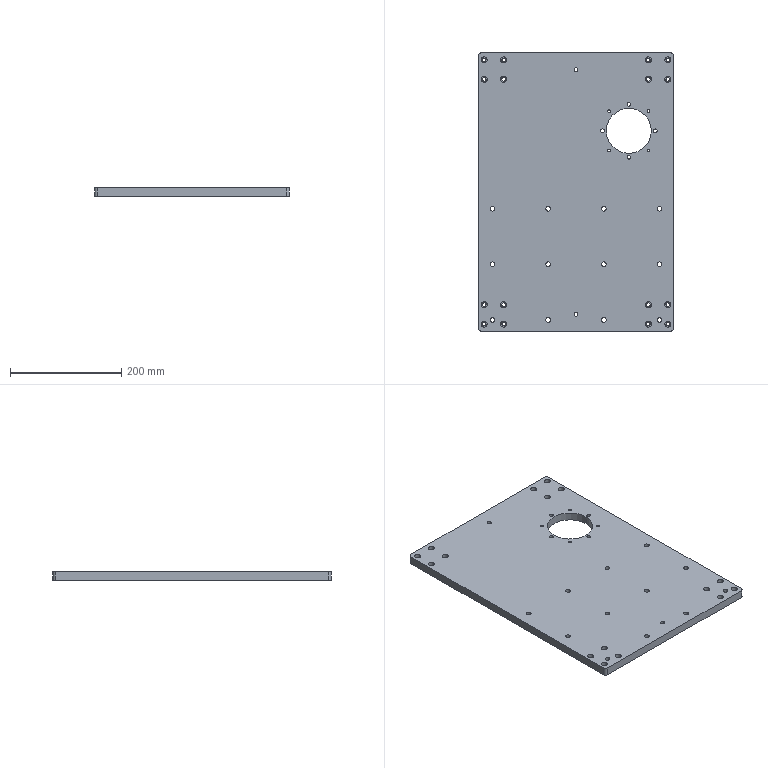NC program | Mastercam | posted with a generic post | part box 350 x 500 x 15 mm
Lines 2013 to 2659 of 4195:
N320 T6 M6
N330 G0 G90 G17 G54 X-202.5 Y-130. A0. S7000 M3
N340 G43 H6 Z50. M8
N350 Z1.
N360 G1 Z0. F600.
N370 X-204.211 Y-130.271 F3000.
N380 G3 X-204.445 Y-130.991 I.991 J-.72
N390 X-203.94 Y-131.982 I1.225 J0.
N400 X-202.5 Y-132.45 Z-.05 I1.44 J1.982
N410 X-200.05 Y-130. Z-.175 I0. J2.45
N420 X-202.5 Y-127.55 Z-.3 I-2.45 J0.
N430 X-204.95 Y-130. Z-.425 I0. J-2.45
N440 X-203.94 Y-131.982 Z-.5 I2.45 J0.
N450 X-202.5 Y-132.45 Z-.55 I1.44 J1.982
N460 X-200.05 Y-130. Z-.675 I0. J2.45
N470 X-202.5 Y-127.55 Z-.8 I-2.45 J0.
N480 X-204.95 Y-130. Z-.925 I0. J-2.45
N490 X-203.94 Y-131.982 Z-1. I2.45 J0.
N500 X-202.5 Y-132.45 Z-1.05 I1.44 J1.982
N510 X-200.05 Y-130. Z-1.175 I0. J2.45
N520 X-202.5 Y-127.55 Z-1.3 I-2.45 J0.
N530 X-204.95 Y-130. Z-1.425 I0. J-2.45
N540 X-203.94 Y-131.982 Z-1.5 I2.45 J0.
N550 X-202.5 Y-132.45 Z-1.55 I1.44 J1.982
N560 X-200.05 Y-130. Z-1.675 I0. J2.45
N570 X-202.5 Y-127.55 Z-1.8 I-2.45 J0.
N580 X-204.95 Y-130. Z-1.925 I0. J-2.45
N590 X-203.94 Y-131.982 Z-2. I2.45 J0.
N600 X-202.5 Y-132.45 Z-2.05 I1.44 J1.982
N610 X-200.05 Y-130. Z-2.175 I0. J2.45
N620 X-202.5 Y-127.55 Z-2.3 I-2.45 J0.
N630 X-204.95 Y-130. Z-2.425 I0. J-2.45
N640 X-203.94 Y-131.982 Z-2.5 I2.45 J0.
N650 X-202.5 Y-132.45 Z-2.55 I1.44 J1.982
N660 X-200.05 Y-130. Z-2.675 I0. J2.45
N670 X-202.5 Y-127.55 Z-2.8 I-2.45 J0.
N680 X-204.95 Y-130. Z-2.925 I0. J-2.45
N690 X-203.94 Y-131.982 Z-3. I2.45 J0.
N700 X-202.5 Y-132.45 Z-3.05 I1.44 J1.982
N710 X-200.05 Y-130. Z-3.175 I0. J2.45
N720 X-202.5 Y-127.55 Z-3.3 I-2.45 J0.
N730 X-204.95 Y-130. Z-3.425 I0. J-2.45
N740 X-203.94 Y-131.982 Z-3.5 I2.45 J0.
N750 X-202.5 Y-132.45 Z-3.55 I1.44 J1.982
N760 X-200.05 Y-130. Z-3.675 I0. J2.45
N770 X-202.5 Y-127.55 Z-3.8 I-2.45 J0.
N780 X-204.95 Y-130. Z-3.925 I0. J-2.45
N790 X-203.94 Y-131.982 Z-4. I2.45 J0.
N800 X-202.5 Y-132.45 Z-4.05 I1.44 J1.982
N810 X-200.05 Y-130. Z-4.175 I0. J2.45
N820 X-202.5 Y-127.55 Z-4.3 I-2.45 J0.
N830 X-204.95 Y-130. Z-4.425 I0. J-2.45
N840 X-203.94 Y-131.982 Z-4.5 I2.45 J0.
N850 X-202.5 Y-132.45 Z-4.55 I1.44 J1.982
N860 X-200.05 Y-130. Z-4.675 I0. J2.45
N870 X-202.5 Y-127.55 Z-4.8 I-2.45 J0.
N880 X-204.95 Y-130. Z-4.925 I0. J-2.45
N890 X-203.94 Y-131.982 Z-5. I2.45 J0.
N900 X-202.5 Y-132.45 Z-5.05 I1.44 J1.982
N910 X-200.05 Y-130. Z-5.175 I0. J2.45
N920 X-202.5 Y-127.55 Z-5.3 I-2.45 J0.
N930 X-204.95 Y-130. Z-5.425 I0. J-2.45
N940 X-203.94 Y-131.982 Z-5.5 I2.45 J0.
N950 X-202.5 Y-132.45 Z-5.55 I1.44 J1.982
N960 X-200.05 Y-130. Z-5.675 I0. J2.45
N970 X-202.5 Y-127.55 Z-5.8 I-2.45 J0.
N980 X-204.95 Y-130. Z-5.925 I0. J-2.45
N990 X-203.94 Y-131.982 Z-6. I2.45 J0.
N1000 X-202.5 Y-132.45 Z-6.05 I1.44 J1.982
N1010 X-200.05 Y-130. Z-6.175 I0. J2.45
N1020 X-202.5 Y-127.55 Z-6.3 I-2.45 J0.
N1030 X-204.95 Y-130. Z-6.425 I0. J-2.45
N1040 X-203.94 Y-131.982 Z-6.5 I2.45 J0.
N1050 X-202.5 Y-132.45 Z-6.55 I1.44 J1.982
N1060 X-200.05 Y-130. Z-6.675 I0. J2.45
N1070 X-202.5 Y-127.55 Z-6.8 I-2.45 J0.
N1080 X-204.95 Y-130. I0. J-2.45 F1500.
N1090 X-202.5 Y-132.45 I2.45 J0.
N1100 X-200.05 Y-130. I0. J2.45
N1110 X-202.5 Y-127.55 I-2.45 J0.
N1120 X-203.725 Y-128.775 I0. J-1.225
N1130 G1 X-202.5 Y-130.
N1140 G0 Z0.
N1150 G1 X-201.25 Y-128.75 F750.
N1160 G3 X-202.5 Y-127.5 I-1.25 J0.
N1170 X-205. Y-130. I0. J-2.5
N1180 X-202.5 Y-132.5 I2.5 J0.
N1190 X-200. Y-130. I0. J2.5
N1200 X-202.5 Y-127.5 I-2.5 J0.
N1210 X-205. Y-130. Z-.5 I0. J-2.5
N1220 X-202.5 Y-132.5 Z-1. I2.5 J0.
N1230 X-200. Y-130. Z-1.5 I0. J2.5
N1240 X-202.5 Y-127.5 Z-2. I-2.5 J0.
N1250 X-205. Y-130. Z-2.5 I0. J-2.5
N1260 X-202.5 Y-132.5 Z-3. I2.5 J0.
N1270 X-200. Y-130. Z-3.5 I0. J2.5
N1280 X-202.5 Y-127.5 Z-4. I-2.5 J0.
N1290 X-205. Y-130. Z-4.5 I0. J-2.5
N1300 X-202.5 Y-132.5 Z-5. I2.5 J0.
N1310 X-200. Y-130. Z-5.5 I0. J2.5
N1320 X-202.5 Y-127.5 Z-6. I-2.5 J0.
N1330 X-205. Y-130. Z-6.5 I0. J-2.5
N1340 X-203.969 Y-132.023 Z-6.8 I2.5 J0.
N1350 X-202.5 Y-132.5 I1.469 J2.023
N1360 X-200. Y-130. I0. J2.5
N1370 X-202.5 Y-127.5 I-2.5 J0.
N1380 X-205. Y-130. I0. J-2.5
N1390 X-203.969 Y-132.023 I2.5 J0.
N1400 X-203.235 Y-132.261 I.734 J1.012
N1410 X-202.223 Y-131.746 I0. J1.25
N1420 G1 X-202.5 Y-130.
N1430 G0 Z50.
N1440 Y-165.
N1450 Z1.
N1460 G1 Z0. F600.
N1470 X-204.211 Y-165.271 F3000.
N1480 G3 X-204.445 Y-165.991 I.991 J-.72
N1490 X-203.94 Y-166.982 I1.225 J0.
N1500 X-202.5 Y-167.45 Z-.05 I1.44 J1.982
N1510 X-200.05 Y-165. Z-.175 I0. J2.45
N1520 X-202.5 Y-162.55 Z-.3 I-2.45 J0.
N1530 X-204.95 Y-165. Z-.425 I0. J-2.45
N1540 X-203.94 Y-166.982 Z-.5 I2.45 J0.
N1550 X-202.5 Y-167.45 Z-.55 I1.44 J1.982
N1560 X-200.05 Y-165. Z-.675 I0. J2.45
N1570 X-202.5 Y-162.55 Z-.8 I-2.45 J0.
N1580 X-204.95 Y-165. Z-.925 I0. J-2.45
N1590 X-203.94 Y-166.982 Z-1. I2.45 J0.
N1600 X-202.5 Y-167.45 Z-1.05 I1.44 J1.982
N1610 X-200.05 Y-165. Z-1.175 I0. J2.45
N1620 X-202.5 Y-162.55 Z-1.3 I-2.45 J0.
N1630 X-204.95 Y-165. Z-1.425 I0. J-2.45
N1640 X-203.94 Y-166.982 Z-1.5 I2.45 J0.
N1650 X-202.5 Y-167.45 Z-1.55 I1.44 J1.982
N1660 X-200.05 Y-165. Z-1.675 I0. J2.45
N1670 X-202.5 Y-162.55 Z-1.8 I-2.45 J0.
N1680 X-204.95 Y-165. Z-1.925 I0. J-2.45
N1690 X-203.94 Y-166.982 Z-2. I2.45 J0.
N1700 X-202.5 Y-167.45 Z-2.05 I1.44 J1.982
N1710 X-200.05 Y-165. Z-2.175 I0. J2.45
N1720 X-202.5 Y-162.55 Z-2.3 I-2.45 J0.
N1730 X-204.95 Y-165. Z-2.425 I0. J-2.45
N1740 X-203.94 Y-166.982 Z-2.5 I2.45 J0.
N1750 X-202.5 Y-167.45 Z-2.55 I1.44 J1.982
N1760 X-200.05 Y-165. Z-2.675 I0. J2.45
N1770 X-202.5 Y-162.55 Z-2.8 I-2.45 J0.
N1780 X-204.95 Y-165. Z-2.925 I0. J-2.45
N1790 X-203.94 Y-166.982 Z-3. I2.45 J0.
N1800 X-202.5 Y-167.45 Z-3.05 I1.44 J1.982
N1810 X-200.05 Y-165. Z-3.175 I0. J2.45
N1820 X-202.5 Y-162.55 Z-3.3 I-2.45 J0.
N1830 X-204.95 Y-165. Z-3.425 I0. J-2.45
N1840 X-203.94 Y-166.982 Z-3.5 I2.45 J0.
N1850 X-202.5 Y-167.45 Z-3.55 I1.44 J1.982
N1860 X-200.05 Y-165. Z-3.675 I0. J2.45
N1870 X-202.5 Y-162.55 Z-3.8 I-2.45 J0.
N1880 X-204.95 Y-165. Z-3.925 I0. J-2.45
N1890 X-203.94 Y-166.982 Z-4. I2.45 J0.
N1900 X-202.5 Y-167.45 Z-4.05 I1.44 J1.982
N1910 X-200.05 Y-165. Z-4.175 I0. J2.45
N1920 X-202.5 Y-162.55 Z-4.3 I-2.45 J0.
N1930 X-204.95 Y-165. Z-4.425 I0. J-2.45
N1940 X-203.94 Y-166.982 Z-4.5 I2.45 J0.
N1950 X-202.5 Y-167.45 Z-4.55 I1.44 J1.982
N1960 X-200.05 Y-165. Z-4.675 I0. J2.45
N1970 X-202.5 Y-162.55 Z-4.8 I-2.45 J0.
N1980 X-204.95 Y-165. Z-4.925 I0. J-2.45
N1990 X-203.94 Y-166.982 Z-5. I2.45 J0.
N2000 X-202.5 Y-167.45 Z-5.05 I1.44 J1.982
N2010 X-200.05 Y-165. Z-5.175 I0. J2.45
N2020 X-202.5 Y-162.55 Z-5.3 I-2.45 J0.
N2030 X-204.95 Y-165. Z-5.425 I0. J-2.45
N2040 X-203.94 Y-166.982 Z-5.5 I2.45 J0.
N2050 X-202.5 Y-167.45 Z-5.55 I1.44 J1.982
N2060 X-200.05 Y-165. Z-5.675 I0. J2.45
N2070 X-202.5 Y-162.55 Z-5.8 I-2.45 J0.
N2080 X-204.95 Y-165. Z-5.925 I0. J-2.45
N2090 X-203.94 Y-166.982 Z-6. I2.45 J0.
N2100 X-202.5 Y-167.45 Z-6.05 I1.44 J1.982
N2110 X-200.05 Y-165. Z-6.175 I0. J2.45
N2120 X-202.5 Y-162.55 Z-6.3 I-2.45 J0.
N2130 X-204.95 Y-165. Z-6.425 I0. J-2.45
N2140 X-203.94 Y-166.982 Z-6.5 I2.45 J0.
N2150 X-202.5 Y-167.45 Z-6.55 I1.44 J1.982
N2160 X-200.05 Y-165. Z-6.675 I0. J2.45
N2170 X-202.5 Y-162.55 Z-6.8 I-2.45 J0.
N2180 X-204.95 Y-165. I0. J-2.45 F1500.
N2190 X-202.5 Y-167.45 I2.45 J0.
N2200 X-200.05 Y-165. I0. J2.45
N2210 X-202.5 Y-162.55 I-2.45 J0.
N2220 X-203.725 Y-163.775 I0. J-1.225
N2230 G1 X-202.5 Y-165.
N2240 G0 Z0.
N2250 G1 X-201.25 Y-163.75 F750.
N2260 G3 X-202.5 Y-162.5 I-1.25 J0.
N2270 X-205. Y-165. I0. J-2.5
N2280 X-202.5 Y-167.5 I2.5 J0.
N2290 X-200. Y-165. I0. J2.5
N2300 X-202.5 Y-162.5 I-2.5 J0.
N2310 X-205. Y-165. Z-.5 I0. J-2.5
N2320 X-202.5 Y-167.5 Z-1. I2.5 J0.
N2330 X-200. Y-165. Z-1.5 I0. J2.5
N2340 X-202.5 Y-162.5 Z-2. I-2.5 J0.
N2350 X-205. Y-165. Z-2.5 I0. J-2.5
N2360 X-202.5 Y-167.5 Z-3. I2.5 J0.
N2370 X-200. Y-165. Z-3.5 I0. J2.5
N2380 X-202.5 Y-162.5 Z-4. I-2.5 J0.
N2390 X-205. Y-165. Z-4.5 I0. J-2.5
N2400 X-202.5 Y-167.5 Z-5. I2.5 J0.
N2410 X-200. Y-165. Z-5.5 I0. J2.5
N2420 X-202.5 Y-162.5 Z-6. I-2.5 J0.
N2430 X-205. Y-165. Z-6.5 I0. J-2.5
N2440 X-203.969 Y-167.023 Z-6.8 I2.5 J0.
N2450 X-202.5 Y-167.5 I1.469 J2.023
N2460 X-200. Y-165. I0. J2.5
N2470 X-202.5 Y-162.5 I-2.5 J0.
N2480 X-205. Y-165. I0. J-2.5
N2490 X-203.969 Y-167.023 I2.5 J0.
N2500 X-203.235 Y-167.261 I.734 J1.012
N2510 X-202.223 Y-166.746 I0. J1.25
N2520 G1 X-202.5 Y-165.
N2530 G0 Z50.
N2540 X-237.5
N2550 Z1.
N2560 G1 Z0. F600.
N2570 X-239.211 Y-165.271 F3000.
N2580 G3 X-239.445 Y-165.991 I.991 J-.72
N2590 X-238.94 Y-166.982 I1.225 J0.
N2600 X-237.5 Y-167.45 Z-.05 I1.44 J1.982
N2610 X-235.05 Y-165. Z-.175 I0. J2.45
N2620 X-237.5 Y-162.55 Z-.3 I-2.45 J0.
N2630 X-239.95 Y-165. Z-.425 I0. J-2.45
N2640 X-238.94 Y-166.982 Z-.5 I2.45 J0.
N2650 X-237.5 Y-167.45 Z-.55 I1.44 J1.982
N2660 X-235.05 Y-165. Z-.675 I0. J2.45
N2670 X-237.5 Y-162.55 Z-.8 I-2.45 J0.
N2680 X-239.95 Y-165. Z-.925 I0. J-2.45
N2690 X-238.94 Y-166.982 Z-1. I2.45 J0.
N2700 X-237.5 Y-167.45 Z-1.05 I1.44 J1.982
N2710 X-235.05 Y-165. Z-1.175 I0. J2.45
N2720 X-237.5 Y-162.55 Z-1.3 I-2.45 J0.
N2730 X-239.95 Y-165. Z-1.425 I0. J-2.45
N2740 X-238.94 Y-166.982 Z-1.5 I2.45 J0.
N2750 X-237.5 Y-167.45 Z-1.55 I1.44 J1.982
N2760 X-235.05 Y-165. Z-1.675 I0. J2.45
N2770 X-237.5 Y-162.55 Z-1.8 I-2.45 J0.
N2780 X-239.95 Y-165. Z-1.925 I0. J-2.45
N2790 X-238.94 Y-166.982 Z-2. I2.45 J0.
N2800 X-237.5 Y-167.45 Z-2.05 I1.44 J1.982
N2810 X-235.05 Y-165. Z-2.175 I0. J2.45
N2820 X-237.5 Y-162.55 Z-2.3 I-2.45 J0.
N2830 X-239.95 Y-165. Z-2.425 I0. J-2.45
N2840 X-238.94 Y-166.982 Z-2.5 I2.45 J0.
N2850 X-237.5 Y-167.45 Z-2.55 I1.44 J1.982
N2860 X-235.05 Y-165. Z-2.675 I0. J2.45
N2870 X-237.5 Y-162.55 Z-2.8 I-2.45 J0.
N2880 X-239.95 Y-165. Z-2.925 I0. J-2.45
N2890 X-238.94 Y-166.982 Z-3. I2.45 J0.
N2900 X-237.5 Y-167.45 Z-3.05 I1.44 J1.982
N2910 X-235.05 Y-165. Z-3.175 I0. J2.45
N2920 X-237.5 Y-162.55 Z-3.3 I-2.45 J0.
N2930 X-239.95 Y-165. Z-3.425 I0. J-2.45
N2940 X-238.94 Y-166.982 Z-3.5 I2.45 J0.
N2950 X-237.5 Y-167.45 Z-3.55 I1.44 J1.982
N2960 X-235.05 Y-165. Z-3.675 I0. J2.45
N2970 X-237.5 Y-162.55 Z-3.8 I-2.45 J0.
N2980 X-239.95 Y-165. Z-3.925 I0. J-2.45
N2990 X-238.94 Y-166.982 Z-4. I2.45 J0.
N3000 X-237.5 Y-167.45 Z-4.05 I1.44 J1.982
N3010 X-235.05 Y-165. Z-4.175 I0. J2.45
N3020 X-237.5 Y-162.55 Z-4.3 I-2.45 J0.
N3030 X-239.95 Y-165. Z-4.425 I0. J-2.45
N3040 X-238.94 Y-166.982 Z-4.5 I2.45 J0.
N3050 X-237.5 Y-167.45 Z-4.55 I1.44 J1.982
N3060 X-235.05 Y-165. Z-4.675 I0. J2.45
N3070 X-237.5 Y-162.55 Z-4.8 I-2.45 J0.
N3080 X-239.95 Y-165. Z-4.925 I0. J-2.45
N3090 X-238.94 Y-166.982 Z-5. I2.45 J0.
N3100 X-237.5 Y-167.45 Z-5.05 I1.44 J1.982
N3110 X-235.05 Y-165. Z-5.175 I0. J2.45
N3120 X-237.5 Y-162.55 Z-5.3 I-2.45 J0.
N3130 X-239.95 Y-165. Z-5.425 I0. J-2.45
N3140 X-238.94 Y-166.982 Z-5.5 I2.45 J0.
N3150 X-237.5 Y-167.45 Z-5.55 I1.44 J1.982
N3160 X-235.05 Y-165. Z-5.675 I0. J2.45
N3170 X-237.5 Y-162.55 Z-5.8 I-2.45 J0.
N3180 X-239.95 Y-165. Z-5.925 I0. J-2.45
N3190 X-238.94 Y-166.982 Z-6. I2.45 J0.
N3200 X-237.5 Y-167.45 Z-6.05 I1.44 J1.982
N3210 X-235.05 Y-165. Z-6.175 I0. J2.45
N3220 X-237.5 Y-162.55 Z-6.3 I-2.45 J0.
N3230 X-239.95 Y-165. Z-6.425 I0. J-2.45
N3240 X-238.94 Y-166.982 Z-6.5 I2.45 J0.
N3250 X-237.5 Y-167.45 Z-6.55 I1.44 J1.982
N3260 X-235.05 Y-165. Z-6.675 I0. J2.45
N3270 X-237.5 Y-162.55 Z-6.8 I-2.45 J0.
N3280 X-239.95 Y-165. I0. J-2.45 F1500.
N3290 X-237.5 Y-167.45 I2.45 J0.
N3300 X-235.05 Y-165. I0. J2.45
N3310 X-237.5 Y-162.55 I-2.45 J0.
N3320 X-238.725 Y-163.775 I0. J-1.225
N3330 G1 X-237.5 Y-165.
N3340 G0 Z0.
N3350 G1 X-236.25 Y-163.75 F750.
N3360 G3 X-237.5 Y-162.5 I-1.25 J0.
N3370 X-240. Y-165. I0. J-2.5
N3380 X-237.5 Y-167.5 I2.5 J0.
N3390 X-235. Y-165. I0. J2.5
N3400 X-237.5 Y-162.5 I-2.5 J0.
N3410 X-240. Y-165. Z-.5 I0. J-2.5
N3420 X-237.5 Y-167.5 Z-1. I2.5 J0.
N3430 X-235. Y-165. Z-1.5 I0. J2.5
N3440 X-237.5 Y-162.5 Z-2. I-2.5 J0.
N3450 X-240. Y-165. Z-2.5 I0. J-2.5
N3460 X-237.5 Y-167.5 Z-3. I2.5 J0.
N3470 X-235. Y-165. Z-3.5 I0. J2.5
N3480 X-237.5 Y-162.5 Z-4. I-2.5 J0.
N3490 X-240. Y-165. Z-4.5 I0. J-2.5
N3500 X-237.5 Y-167.5 Z-5. I2.5 J0.
N3510 X-235. Y-165. Z-5.5 I0. J2.5
N3520 X-237.5 Y-162.5 Z-6. I-2.5 J0.
N3530 X-240. Y-165. Z-6.5 I0. J-2.5
N3540 X-238.969 Y-167.023 Z-6.8 I2.5 J0.
N3550 X-237.5 Y-167.5 I1.469 J2.023
N3560 X-235. Y-165. I0. J2.5
N3570 X-237.5 Y-162.5 I-2.5 J0.
N3580 X-240. Y-165. I0. J-2.5
N3590 X-238.969 Y-167.023 I2.5 J0.
N3600 X-238.235 Y-167.261 I.734 J1.012
N3610 X-237.223 Y-166.746 I0. J1.25
N3620 G1 X-237.5 Y-165.
N3630 G0 Z50.
N3640 Y-130.
N3650 Z1.
N3660 G1 Z0. F600.
N3670 X-239.211 Y-130.271 F3000.
N3680 G3 X-239.445 Y-130.991 I.991 J-.72
N3690 X-238.94 Y-131.982 I1.225 J0.
N3700 X-237.5 Y-132.45 Z-.05 I1.44 J1.982
N3710 X-235.05 Y-130. Z-.175 I0. J2.45
N3720 X-237.5 Y-127.55 Z-.3 I-2.45 J0.
N3730 X-239.95 Y-130. Z-.425 I0. J-2.45
N3740 X-238.94 Y-131.982 Z-.5 I2.45 J0.
N3750 X-237.5 Y-132.45 Z-.55 I1.44 J1.982
N3760 X-235.05 Y-130. Z-.675 I0. J2.45
N3770 X-237.5 Y-127.55 Z-.8 I-2.45 J0.
N3780 X-239.95 Y-130. Z-.925 I0. J-2.45
N3790 X-238.94 Y-131.982 Z-1. I2.45 J0.
N3800 X-237.5 Y-132.45 Z-1.05 I1.44 J1.982
N3810 X-235.05 Y-130. Z-1.175 I0. J2.45
N3820 X-237.5 Y-127.55 Z-1.3 I-2.45 J0.
N3830 X-239.95 Y-130. Z-1.425 I0. J-2.45
N3840 X-238.94 Y-131.982 Z-1.5 I2.45 J0.
N3850 X-237.5 Y-132.45 Z-1.55 I1.44 J1.982
N3860 X-235.05 Y-130. Z-1.675 I0. J2.45
N3870 X-237.5 Y-127.55 Z-1.8 I-2.45 J0.
N3880 X-239.95 Y-130. Z-1.925 I0. J-2.45
N3890 X-238.94 Y-131.982 Z-2. I2.45 J0.
N3900 X-237.5 Y-132.45 Z-2.05 I1.44 J1.982
N3910 X-235.05 Y-130. Z-2.175 I0. J2.45
N3920 X-237.5 Y-127.55 Z-2.3 I-2.45 J0.
N3930 X-239.95 Y-130. Z-2.425 I0. J-2.45
N3940 X-238.94 Y-131.982 Z-2.5 I2.45 J0.
N3950 X-237.5 Y-132.45 Z-2.55 I1.44 J1.982
N3960 X-235.05 Y-130. Z-2.675 I0. J2.45
N3970 X-237.5 Y-127.55 Z-2.8 I-2.45 J0.
N3980 X-239.95 Y-130. Z-2.925 I0. J-2.45
N3990 X-238.94 Y-131.982 Z-3. I2.45 J0.
N4000 X-237.5 Y-132.45 Z-3.05 I1.44 J1.982
N4010 X-235.05 Y-130. Z-3.175 I0. J2.45
N4020 X-237.5 Y-127.55 Z-3.3 I-2.45 J0.
N4030 X-239.95 Y-130. Z-3.425 I0. J-2.45
N4040 X-238.94 Y-131.982 Z-3.5 I2.45 J0.
N4050 X-237.5 Y-132.45 Z-3.55 I1.44 J1.982
N4060 X-235.05 Y-130. Z-3.675 I0. J2.45
N4070 X-237.5 Y-127.55 Z-3.8 I-2.45 J0.
N4080 X-239.95 Y-130. Z-3.925 I0. J-2.45
N4090 X-238.94 Y-131.982 Z-4. I2.45 J0.
N4100 X-237.5 Y-132.45 Z-4.05 I1.44 J1.982
N4110 X-235.05 Y-130. Z-4.175 I0. J2.45
N4120 X-237.5 Y-127.55 Z-4.3 I-2.45 J0.
N4130 X-239.95 Y-130. Z-4.425 I0. J-2.45
N4140 X-238.94 Y-131.982 Z-4.5 I2.45 J0.
N4150 X-237.5 Y-132.45 Z-4.55 I1.44 J1.982
N4160 X-235.05 Y-130. Z-4.675 I0. J2.45
N4170 X-237.5 Y-127.55 Z-4.8 I-2.45 J0.
N4180 X-239.95 Y-130. Z-4.925 I0. J-2.45
N4190 X-238.94 Y-131.982 Z-5. I2.45 J0.
N4200 X-237.5 Y-132.45 Z-5.05 I1.44 J1.982
N4210 X-235.05 Y-130. Z-5.175 I0. J2.45
N4220 X-237.5 Y-127.55 Z-5.3 I-2.45 J0.
N4230 X-239.95 Y-130. Z-5.425 I0. J-2.45
N4240 X-238.94 Y-131.982 Z-5.5 I2.45 J0.
N4250 X-237.5 Y-132.45 Z-5.55 I1.44 J1.982
N4260 X-235.05 Y-130. Z-5.675 I0. J2.45
N4270 X-237.5 Y-127.55 Z-5.8 I-2.45 J0.
N4280 X-239.95 Y-130. Z-5.925 I0. J-2.45
N4290 X-238.94 Y-131.982 Z-6. I2.45 J0.
N4300 X-237.5 Y-132.45 Z-6.05 I1.44 J1.982
N4310 X-235.05 Y-130. Z-6.175 I0. J2.45
N4320 X-237.5 Y-127.55 Z-6.3 I-2.45 J0.
N4330 X-239.95 Y-130. Z-6.425 I0. J-2.45
N4340 X-238.94 Y-131.982 Z-6.5 I2.45 J0.
N4350 X-237.5 Y-132.45 Z-6.55 I1.44 J1.982
N4360 X-235.05 Y-130. Z-6.675 I0. J2.45
N4370 X-237.5 Y-127.55 Z-6.8 I-2.45 J0.
N4380 X-239.95 Y-130. I0. J-2.45 F1500.
N4390 X-237.5 Y-132.45 I2.45 J0.
N4400 X-235.05 Y-130. I0. J2.45
N4410 X-237.5 Y-127.55 I-2.45 J0.
N4420 X-238.725 Y-128.775 I0. J-1.225
N4430 G1 X-237.5 Y-130.
N4440 G0 Z0.
N4450 G1 X-236.25 Y-128.75 F750.
N4460 G3 X-237.5 Y-127.5 I-1.25 J0.
N4470 X-240. Y-130. I0. J-2.5
N4480 X-237.5 Y-132.5 I2.5 J0.
N4490 X-235. Y-130. I0. J2.5
N4500 X-237.5 Y-127.5 I-2.5 J0.
N4510 X-240. Y-130. Z-.5 I0. J-2.5
N4520 X-237.5 Y-132.5 Z-1. I2.5 J0.
N4530 X-235. Y-130. Z-1.5 I0. J2.5
N4540 X-237.5 Y-127.5 Z-2. I-2.5 J0.
N4550 X-240. Y-130. Z-2.5 I0. J-2.5
N4560 X-237.5 Y-132.5 Z-3. I2.5 J0.
N4570 X-235. Y-130. Z-3.5 I0. J2.5
N4580 X-237.5 Y-127.5 Z-4. I-2.5 J0.
N4590 X-240. Y-130. Z-4.5 I0. J-2.5
N4600 X-237.5 Y-132.5 Z-5. I2.5 J0.
N4610 X-235. Y-130. Z-5.5 I0. J2.5
N4620 X-237.5 Y-127.5 Z-6. I-2.5 J0.
N4630 X-240. Y-130. Z-6.5 I0. J-2.5
N4640 X-238.969 Y-132.023 Z-6.8 I2.5 J0.
N4650 X-237.5 Y-132.5 I1.469 J2.023
N4660 X-235. Y-130. I0. J2.5
N4670 X-237.5 Y-127.5 I-2.5 J0.
N4680 X-240. Y-130. I0. J-2.5
N4690 X-238.969 Y-132.023 I2.5 J0.
N4700 X-238.235 Y-132.261 I.734 J1.012
N4710 X-237.223 Y-131.746 I0. J1.25
N4720 G1 X-237.5 Y-130.
N4730 G0 Z50.
N4740 Y130.
N4750 Z1.
N4760 G1 Z0. F600.
N4770 X-239.211 Y129.729 F3000.
N4780 G3 X-239.445 Y129.009 I.991 J-.72
N4790 X-238.94 Y128.018 I1.225 J0.
N4800 X-237.5 Y127.55 Z-.05 I1.44 J1.982
N4810 X-235.05 Y130. Z-.175 I0. J2.45
N4820 X-237.5 Y132.45 Z-.3 I-2.45 J0.
N4830 X-239.95 Y130. Z-.425 I0. J-2.45
N4840 X-238.94 Y128.018 Z-.5 I2.45 J0.
N4850 X-237.5 Y127.55 Z-.55 I1.44 J1.982
N4860 X-235.05 Y130. Z-.675 I0. J2.45
N4870 X-237.5 Y132.45 Z-.8 I-2.45 J0.
N4880 X-239.95 Y130. Z-.925 I0. J-2.45
N4890 X-238.94 Y128.018 Z-1. I2.45 J0.
N4900 X-237.5 Y127.55 Z-1.05 I1.44 J1.982
N4910 X-235.05 Y130. Z-1.175 I0. J2.45
N4920 X-237.5 Y132.45 Z-1.3 I-2.45 J0.
N4930 X-239.95 Y130. Z-1.425 I0. J-2.45
N4940 X-238.94 Y128.018 Z-1.5 I2.45 J0.
N4950 X-237.5 Y127.55 Z-1.55 I1.44 J1.982
N4960 X-235.05 Y130. Z-1.675 I0. J2.45
N4970 X-237.5 Y132.45 Z-1.8 I-2.45 J0.
N4980 X-239.95 Y130. Z-1.925 I0. J-2.45
N4990 X-238.94 Y128.018 Z-2. I2.45 J0.
N5000 X-237.5 Y127.55 Z-2.05 I1.44 J1.982
N5010 X-235.05 Y130. Z-2.175 I0. J2.45
N5020 X-237.5 Y132.45 Z-2.3 I-2.45 J0.
N5030 X-239.95 Y130. Z-2.425 I0. J-2.45
N5040 X-238.94 Y128.018 Z-2.5 I2.45 J0.
N5050 X-237.5 Y127.55 Z-2.55 I1.44 J1.982
N5060 X-235.05 Y130. Z-2.675 I0. J2.45
N5070 X-237.5 Y132.45 Z-2.8 I-2.45 J0.
N5080 X-239.95 Y130. Z-2.925 I0. J-2.45
N5090 X-238.94 Y128.018 Z-3. I2.45 J0.
N5100 X-237.5 Y127.55 Z-3.05 I1.44 J1.982
N5110 X-235.05 Y130. Z-3.175 I0. J2.45
N5120 X-237.5 Y132.45 Z-3.3 I-2.45 J0.
N5130 X-239.95 Y130. Z-3.425 I0. J-2.45
N5140 X-238.94 Y128.018 Z-3.5 I2.45 J0.
N5150 X-237.5 Y127.55 Z-3.55 I1.44 J1.982
N5160 X-235.05 Y130. Z-3.675 I0. J2.45
N5170 X-237.5 Y132.45 Z-3.8 I-2.45 J0.
N5180 X-239.95 Y130. Z-3.925 I0. J-2.45
N5190 X-238.94 Y128.018 Z-4. I2.45 J0.
N5200 X-237.5 Y127.55 Z-4.05 I1.44 J1.982
N5210 X-235.05 Y130. Z-4.175 I0. J2.45
N5220 X-237.5 Y132.45 Z-4.3 I-2.45 J0.
N5230 X-239.95 Y130. Z-4.425 I0. J-2.45
N5240 X-238.94 Y128.018 Z-4.5 I2.45 J0.
N5250 X-237.5 Y127.55 Z-4.55 I1.44 J1.982
N5260 X-235.05 Y130. Z-4.675 I0. J2.45
N5270 X-237.5 Y132.45 Z-4.8 I-2.45 J0.
N5280 X-239.95 Y130. Z-4.925 I0. J-2.45
N5290 X-238.94 Y128.018 Z-5. I2.45 J0.
N5300 X-237.5 Y127.55 Z-5.05 I1.44 J1.982
N5310 X-235.05 Y130. Z-5.175 I0. J2.45
N5320 X-237.5 Y132.45 Z-5.3 I-2.45 J0.
N5330 X-239.95 Y130. Z-5.425 I0. J-2.45
N5340 X-238.94 Y128.018 Z-5.5 I2.45 J0.
N5350 X-237.5 Y127.55 Z-5.55 I1.44 J1.982
N5360 X-235.05 Y130. Z-5.675 I0. J2.45
N5370 X-237.5 Y132.45 Z-5.8 I-2.45 J0.
N5380 X-239.95 Y130. Z-5.925 I0. J-2.45
N5390 X-238.94 Y128.018 Z-6. I2.45 J0.
N5400 X-237.5 Y127.55 Z-6.05 I1.44 J1.982
N5410 X-235.05 Y130. Z-6.175 I0. J2.45
N5420 X-237.5 Y132.45 Z-6.3 I-2.45 J0.
N5430 X-239.95 Y130. Z-6.425 I0. J-2.45
N5440 X-238.94 Y128.018 Z-6.5 I2.45 J0.
N5450 X-237.5 Y127.55 Z-6.55 I1.44 J1.982
N5460 X-235.05 Y130. Z-6.675 I0. J2.45
N5470 X-237.5 Y132.45 Z-6.8 I-2.45 J0.
N5480 X-239.95 Y130. I0. J-2.45 F1500.
N5490 X-237.5 Y127.55 I2.45 J0.
N5500 X-235.05 Y130. I0. J2.45
N5510 X-237.5 Y132.45 I-2.45 J0.
N5520 X-238.725 Y131.225 I0. J-1.225
N5530 G1 X-237.5 Y130.
N5540 G0 Z0.
N5550 G1 X-236.25 Y131.25 F750.
N5560 G3 X-237.5 Y132.5 I-1.25 J0.
N5570 X-240. Y130. I0. J-2.5
N5580 X-237.5 Y127.5 I2.5 J0.
N5590 X-235. Y130. I0. J2.5
N5600 X-237.5 Y132.5 I-2.5 J0.
N5610 X-240. Y130. Z-.5 I0. J-2.5
N5620 X-237.5 Y127.5 Z-1. I2.5 J0.
N5630 X-235. Y130. Z-1.5 I0. J2.5
N5640 X-237.5 Y132.5 Z-2. I-2.5 J0.
N5650 X-240. Y130. Z-2.5 I0. J-2.5
N5660 X-237.5 Y127.5 Z-3. I2.5 J0.
N5670 X-235. Y130. Z-3.5 I0. J2.5
N5680 X-237.5 Y132.5 Z-4. I-2.5 J0.
N5690 X-240. Y130. Z-4.5 I0. J-2.5
N5700 X-237.5 Y127.5 Z-5. I2.5 J0.
N5710 X-235. Y130. Z-5.5 I0. J2.5
N5720 X-237.5 Y132.5 Z-6. I-2.5 J0.
N5730 X-240. Y130. Z-6.5 I0. J-2.5
N5740 X-238.969 Y127.977 Z-6.8 I2.5 J0.
N5750 X-237.5 Y127.5 I1.469 J2.023
N5760 X-235. Y130. I0. J2.5
N5770 X-237.5 Y132.5 I-2.5 J0.
N5780 X-240. Y130. I0. J-2.5
N5790 X-238.969 Y127.977 I2.5 J0.
N5800 X-238.235 Y127.739 I.734 J1.012
N5810 X-237.223 Y128.254 I0. J1.25
N5820 G1 X-237.5 Y130.
N5830 G0 Z50.
N5840 Y165.
N5850 Z1.
N5860 G1 Z0. F600.
N5870 X-239.211 Y164.729 F3000.
N5880 G3 X-239.445 Y164.009 I.991 J-.72
N5890 X-238.94 Y163.018 I1.225 J0.
N5900 X-237.5 Y162.55 Z-.05 I1.44 J1.982
N5910 X-235.05 Y165. Z-.175 I0. J2.45
N5920 X-237.5 Y167.45 Z-.3 I-2.45 J0.
N5930 X-239.95 Y165. Z-.425 I0. J-2.45
N5940 X-238.94 Y163.018 Z-.5 I2.45 J0.
N5950 X-237.5 Y162.55 Z-.55 I1.44 J1.982
N5960 X-235.05 Y165. Z-.675 I0. J2.45
N5970 X-237.5 Y167.45 Z-.8 I-2.45 J0.
N5980 X-239.95 Y165. Z-.925 I0. J-2.45
N5990 X-238.94 Y163.018 Z-1. I2.45 J0.
N6000 X-237.5 Y162.55 Z-1.05 I1.44 J1.982
N6010 X-235.05 Y165. Z-1.175 I0. J2.45
N6020 X-237.5 Y167.45 Z-1.3 I-2.45 J0.
N6030 X-239.95 Y165. Z-1.425 I0. J-2.45
N6040 X-238.94 Y163.018 Z-1.5 I2.45 J0.
N6050 X-237.5 Y162.55 Z-1.55 I1.44 J1.982
N6060 X-235.05 Y165. Z-1.675 I0. J2.45
N6070 X-237.5 Y167.45 Z-1.8 I-2.45 J0.
N6080 X-239.95 Y165. Z-1.925 I0. J-2.45
N6090 X-238.94 Y163.018 Z-2. I2.45 J0.
N6100 X-237.5 Y162.55 Z-2.05 I1.44 J1.982
N6110 X-235.05 Y165. Z-2.175 I0. J2.45
N6120 X-237.5 Y167.45 Z-2.3 I-2.45 J0.
N6130 X-239.95 Y165. Z-2.425 I0. J-2.45
N6140 X-238.94 Y163.018 Z-2.5 I2.45 J0.
N6150 X-237.5 Y162.55 Z-2.55 I1.44 J1.982
N6160 X-235.05 Y165. Z-2.675 I0. J2.45
N6170 X-237.5 Y167.45 Z-2.8 I-2.45 J0.
N6180 X-239.95 Y165. Z-2.925 I0. J-2.45
N6190 X-238.94 Y163.018 Z-3. I2.45 J0.
N6200 X-237.5 Y162.55 Z-3.05 I1.44 J1.982
N6210 X-235.05 Y165. Z-3.175 I0. J2.45
N6220 X-237.5 Y167.45 Z-3.3 I-2.45 J0.
N6230 X-239.95 Y165. Z-3.425 I0. J-2.45
N6240 X-238.94 Y163.018 Z-3.5 I2.45 J0.
N6250 X-237.5 Y162.55 Z-3.55 I1.44 J1.982
N6260 X-235.05 Y165. Z-3.675 I0. J2.45
N6270 X-237.5 Y167.45 Z-3.8 I-2.45 J0.
N6280 X-239.95 Y165. Z-3.925 I0. J-2.45
N6290 X-238.94 Y163.018 Z-4. I2.45 J0.
N6300 X-237.5 Y162.55 Z-4.05 I1.44 J1.982
N6310 X-235.05 Y165. Z-4.175 I0. J2.45
N6320 X-237.5 Y167.45 Z-4.3 I-2.45 J0.
N6330 X-239.95 Y165. Z-4.425 I0. J-2.45
N6340 X-238.94 Y163.018 Z-4.5 I2.45 J0.
N6350 X-237.5 Y162.55 Z-4.55 I1.44 J1.982
N6360 X-235.05 Y165. Z-4.675 I0. J2.45
N6370 X-237.5 Y167.45 Z-4.8 I-2.45 J0.
N6380 X-239.95 Y165. Z-4.925 I0. J-2.45
N6390 X-238.94 Y163.018 Z-5. I2.45 J0.
N6400 X-237.5 Y162.55 Z-5.05 I1.44 J1.982
N6410 X-235.05 Y165. Z-5.175 I0. J2.45
N6420 X-237.5 Y167.45 Z-5.3 I-2.45 J0.
N6430 X-239.95 Y165. Z-5.425 I0. J-2.45
N6440 X-238.94 Y163.018 Z-5.5 I2.45 J0.
N6450 X-237.5 Y162.55 Z-5.55 I1.44 J1.982
N6460 X-235.05 Y165. Z-5.675 I0. J2.45
N6470 X-237.5 Y167.45 Z-5.8 I-2.45 J0.
N6480 X-239.95 Y165. Z-5.925 I0. J-2.45
N6490 X-238.94 Y163.018 Z-6. I2.45 J0.
N6500 X-237.5 Y162.55 Z-6.05 I1.44 J1.982
N6510 X-235.05 Y165. Z-6.175 I0. J2.45
N6520 X-237.5 Y167.45 Z-6.3 I-2.45 J0.
N6530 X-239.95 Y165. Z-6.425 I0. J-2.45
N6540 X-238.94 Y163.018 Z-6.5 I2.45 J0.
N6550 X-237.5 Y162.55 Z-6.55 I1.44 J1.982
N6560 X-235.05 Y165. Z-6.675 I0. J2.45
N6570 X-237.5 Y167.45 Z-6.8 I-2.45 J0.
N6580 X-239.95 Y165. I0. J-2.45 F1500.
N6590 X-237.5 Y162.55 I2.45 J0.
N6600 X-235.05 Y165. I0. J2.45
N6610 X-237.5 Y167.45 I-2.45 J0.
N6620 X-238.725 Y166.225 I0. J-1.225
N6630 G1 X-237.5 Y165.
N6640 G0 Z0.
N6650 G1 X-236.25 Y166.25 F750.
N6660 G3 X-237.5 Y167.5 I-1.25 J0.
N6670 X-240. Y165. I0. J-2.5
N6680 X-237.5 Y162.5 I2.5 J0.
N6690 X-235. Y165. I0. J2.5
N6700 X-237.5 Y167.5 I-2.5 J0.
N6710 X-240. Y165. Z-.5 I0. J-2.5
N6720 X-237.5 Y162.5 Z-1. I2.5 J0.
N6730 X-235. Y165. Z-1.5 I0. J2.5
N6740 X-237.5 Y167.5 Z-2. I-2.5 J0.
N6750 X-240. Y165. Z-2.5 I0. J-2.5
N6760 X-237.5 Y162.5 Z-3. I2.5 J0.
N6770 X-235. Y165. Z-3.5 I0. J2.5
N6780 X-237.5 Y167.5 Z-4. I-2.5 J0.